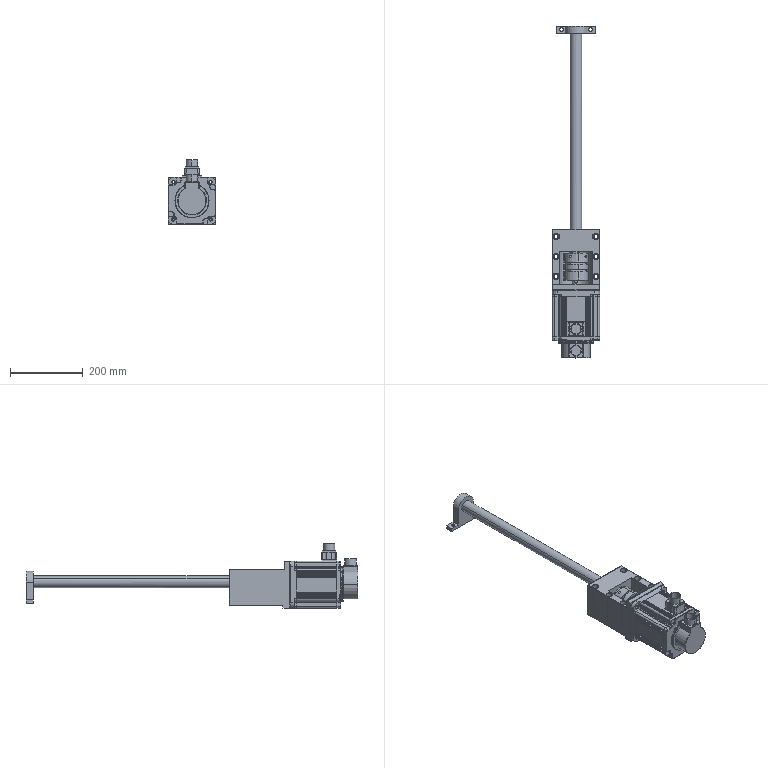Part | SolidWorks | 47 solids | 1219 faces | box 130 x 914.5 x 177.75 mm | volume 425497 mm3 | plane 482 | cylinder 281 | spline 268 | cone 173 | torus 14 | sphere 1 | commonest cylinder face diameters 2 x76 5 x12 10 x12 11 x12 17.5 x12 1 x10